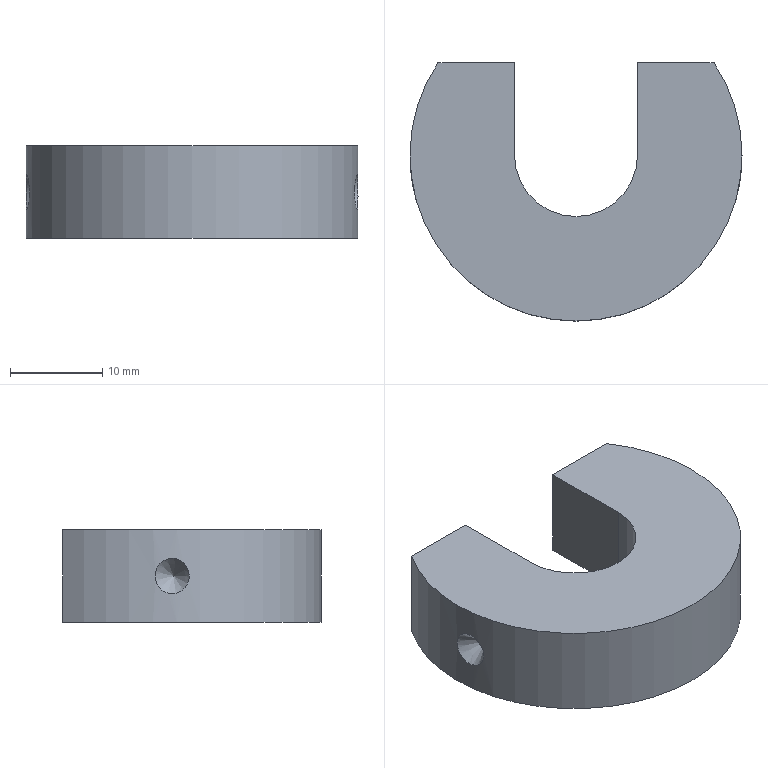Part | NX | features DATUM_CSYS 4, CONE 2, SKETCH 2, EXTRUDE 1, MIRROR_SET 1 | 1 solid | 10 faces | box 36.001 x 28 x 10 mm | volume 6442 mm3 | plane 6 | cylinder 2 | cone 2 | commonest cylinder face diameters 13.349 x1 36 x1
STEP:
#1=CARTESIAN_POINT('',(17.755,-2.958,3.471));
#2=VERTEX_POINT('',#1);
#3=CARTESIAN_POINT('',(17.578,-3.865,4.697));
#4=CARTESIAN_POINT('',(17.749,-3.086,3.311));
#5=CARTESIAN_POINT('',(17.958,-1.543,2.887));
#6=CARTESIAN_POINT('',(18.006,-0.1872,3.755));
#7=CARTESIAN_POINT('',(17.997,0.1688,5.305));
#8=CARTESIAN_POINT('',(18.004,-0.6057,6.698));
#9=CARTESIAN_POINT('',(17.894,-2.162,7.108));
#10=CARTESIAN_POINT('',(17.663,-3.5,6.241));
#11=CARTESIAN_POINT('',(17.578,-3.865,4.697));
#12=CARTESIAN_POINT('',(17.749,-3.086,3.311));
#13=CARTESIAN_POINT('',(17.958,-1.543,2.887));
#14=B_SPLINE_CURVE_WITH_KNOTS('',3,(#3,#4,#5,#6,#7,#8,#9,#10,#11,#12,#13),.UNSPECIFIED.,.T.,.F.,(1,1,1,1,1,1,1,1,1,1,1,1,1,1,1),(-0.00444,-0.00296,-0.00148,0.,0.00148,0.00296,0.00444,0.00592,0.0074,0.00888,0.01036,0.01184,0.01332,0.0148,0.01628),.UNSPECIFIED.);
#15=EDGE_CURVE('',#2,#2,#14,.T.);
#16=ORIENTED_EDGE('',*,*,#15,.F.);
#17=EDGE_LOOP('',(#16));
#18=FACE_BOUND('',#17,.T.);
#19=CARTESIAN_POINT('',(-17.755,-2.958,3.471));
#20=VERTEX_POINT('',#19);
#21=CARTESIAN_POINT('',(-17.958,-1.541,2.887));
#22=CARTESIAN_POINT('',(-17.748,-3.086,3.311));
#23=CARTESIAN_POINT('',(-17.578,-3.865,4.696));
#24=CARTESIAN_POINT('',(-17.663,-3.5,6.241));
#25=CARTESIAN_POINT('',(-17.893,-2.167,7.107));
#26=CARTESIAN_POINT('',(-18.004,-0.6063,6.7));
#27=CARTESIAN_POINT('',(-17.997,0.1689,5.305));
#28=CARTESIAN_POINT('',(-18.006,-0.1867,3.757));
#29=CARTESIAN_POINT('',(-17.958,-1.541,2.887));
#30=CARTESIAN_POINT('',(-17.748,-3.086,3.311));
#31=CARTESIAN_POINT('',(-17.578,-3.865,4.696));
#32=B_SPLINE_CURVE_WITH_KNOTS('',3,(#21,#22,#23,#24,#25,#26,#27,#28,#29,#30,#31),.UNSPECIFIED.,.T.,.F.,(1,1,1,1,1,1,1,1,1,1,1,1,1,1,1),(-0.004442,-0.002961,-0.001481,0.,0.001481,0.002961,0.004442,0.005922,0.007403,0.008884,0.01036,0.01184,0.01333,0.01481,0.01629),.UNSPECIFIED.);
#33=EDGE_CURVE('',#20,#20,#32,.T.);
#34=ORIENTED_EDGE('',*,*,#33,.F.);
#35=EDGE_LOOP('',(#34));
#36=FACE_BOUND('',#35,.T.);
#37=CARTESIAN_POINT('',(14.966,10.,0.));
#38=VERTEX_POINT('',#37);
#39=CARTESIAN_POINT('',(-14.966,10.,0.));
#40=VERTEX_POINT('',#39);
#41=CARTESIAN_POINT('',(0.,0.,0.));
#42=DIRECTION('',(0.,0.,-1.));
#43=DIRECTION('',(1.,0.,0.));
#44=AXIS2_PLACEMENT_3D('',#41,#42,#43);
#45=CIRCLE('',#44,18.);
#46=EDGE_CURVE('',#38,#40,#45,.T.);
#47=ORIENTED_EDGE('',*,*,#46,.F.);
#48=CARTESIAN_POINT('',(14.966,10.,10.));
#49=VERTEX_POINT('',#48);
#50=CARTESIAN_POINT('',(14.966,10.,10.));
#51=DIRECTION('',(0.,0.,-1.));
#52=VECTOR('',#51,1000.);
#53=LINE('',#50,#52);
#54=EDGE_CURVE('',#49,#38,#53,.T.);
#55=ORIENTED_EDGE('',*,*,#54,.F.);
#56=CARTESIAN_POINT('',(-14.966,10.,10.));
#57=VERTEX_POINT('',#56);
#58=CARTESIAN_POINT('',(0.,0.,10.));
#59=DIRECTION('',(0.,0.,-1.));
#60=DIRECTION('',(1.,0.,0.));
#61=AXIS2_PLACEMENT_3D('',#58,#59,#60);
#62=CIRCLE('',#61,18.);
#63=EDGE_CURVE('',#49,#57,#62,.T.);
#64=ORIENTED_EDGE('',*,*,#63,.T.);
#65=CARTESIAN_POINT('',(-14.966,10.,10.));
#66=DIRECTION('',(0.,0.,-1.));
#67=VECTOR('',#66,1000.);
#68=LINE('',#65,#67);
#69=EDGE_CURVE('',#57,#40,#68,.T.);
#70=ORIENTED_EDGE('',*,*,#69,.T.);
#71=EDGE_LOOP('',(#47,#55,#64,#70));
#72=FACE_BOUND('',#71,.T.);
#73=CARTESIAN_POINT('',(0.,0.,10.));
#74=DIRECTION('',(0.,0.,-1.));
#75=DIRECTION('',(-1.,0.,0.));
#76=AXIS2_PLACEMENT_3D('',#73,#74,#75);
#77=CYLINDRICAL_SURFACE('',#76,18.);
#78=ADVANCED_FACE('',(#18,#36,#72),#77,.T.);
#79=CARTESIAN_POINT('',(-6.675,10.,0.));
#80=VERTEX_POINT('',#79);
#81=CARTESIAN_POINT('',(-14.966,10.,0.));
#82=DIRECTION('',(1.,0.,0.));
#83=VECTOR('',#82,1000.);
#84=LINE('',#81,#83);
#85=EDGE_CURVE('',#40,#80,#84,.T.);
#86=ORIENTED_EDGE('',*,*,#85,.F.);
#87=ORIENTED_EDGE('',*,*,#69,.F.);
#88=CARTESIAN_POINT('',(-6.675,10.,10.));
#89=VERTEX_POINT('',#88);
#90=CARTESIAN_POINT('',(-14.966,10.,10.));
#91=DIRECTION('',(1.,0.,0.));
#92=VECTOR('',#91,1000.);
#93=LINE('',#90,#92);
#94=EDGE_CURVE('',#57,#89,#93,.T.);
#95=ORIENTED_EDGE('',*,*,#94,.T.);
#96=CARTESIAN_POINT('',(-6.675,10.,10.));
#97=DIRECTION('',(0.,0.,-1.));
#98=VECTOR('',#97,1000.);
#99=LINE('',#96,#98);
#100=EDGE_CURVE('',#89,#80,#99,.T.);
#101=ORIENTED_EDGE('',*,*,#100,.T.);
#102=EDGE_LOOP('',(#86,#87,#95,#101));
#103=FACE_BOUND('',#102,.T.);
#104=CARTESIAN_POINT('',(-14.966,10.,10.));
#105=DIRECTION('',(0.,1.,0.));
#106=DIRECTION('',(0.,0.,1.));
#107=AXIS2_PLACEMENT_3D('',#104,#105,#106);
#108=PLANE('',#107);
#109=ADVANCED_FACE('',(#103),#108,.T.);
#110=CARTESIAN_POINT('',(-6.675,0.,0.));
#111=VERTEX_POINT('',#110);
#112=CARTESIAN_POINT('',(-6.675,10.,0.));
#113=DIRECTION('',(0.,-1.,0.));
#114=VECTOR('',#113,1000.);
#115=LINE('',#112,#114);
#116=EDGE_CURVE('',#80,#111,#115,.T.);
#117=ORIENTED_EDGE('',*,*,#116,.F.);
#118=ORIENTED_EDGE('',*,*,#100,.F.);
#119=CARTESIAN_POINT('',(-6.675,0.,10.));
#120=VERTEX_POINT('',#119);
#121=CARTESIAN_POINT('',(-6.675,10.,10.));
#122=DIRECTION('',(0.,-1.,0.));
#123=VECTOR('',#122,1000.);
#124=LINE('',#121,#123);
#125=EDGE_CURVE('',#89,#120,#124,.T.);
#126=ORIENTED_EDGE('',*,*,#125,.T.);
#127=CARTESIAN_POINT('',(-6.675,0.,10.));
#128=DIRECTION('',(0.,0.,-1.));
#129=VECTOR('',#128,1000.);
#130=LINE('',#127,#129);
#131=EDGE_CURVE('',#120,#111,#130,.T.);
#132=ORIENTED_EDGE('',*,*,#131,.T.);
#133=EDGE_LOOP('',(#117,#118,#126,#132));
#134=FACE_BOUND('',#133,.T.);
#135=CARTESIAN_POINT('',(-6.675,10.,10.));
#136=DIRECTION('',(1.,0.,0.));
#137=DIRECTION('',(0.,1.,0.));
#138=AXIS2_PLACEMENT_3D('',#135,#136,#137);
#139=PLANE('',#138);
#140=ADVANCED_FACE('',(#134),#139,.T.);
#141=CARTESIAN_POINT('',(6.675,0.,0.));
#142=VERTEX_POINT('',#141);
#143=CARTESIAN_POINT('',(0.,0.,0.));
#144=DIRECTION('',(0.,0.,1.));
#145=DIRECTION('',(1.,0.,0.));
#146=AXIS2_PLACEMENT_3D('',#143,#144,#145);
#147=CIRCLE('',#146,6.675);
#148=EDGE_CURVE('',#111,#142,#147,.T.);
#149=ORIENTED_EDGE('',*,*,#148,.F.);
#150=ORIENTED_EDGE('',*,*,#131,.F.);
#151=CARTESIAN_POINT('',(6.675,0.,10.));
#152=VERTEX_POINT('',#151);
#153=CARTESIAN_POINT('',(0.,0.,10.));
#154=DIRECTION('',(0.,0.,1.));
#155=DIRECTION('',(1.,0.,0.));
#156=AXIS2_PLACEMENT_3D('',#153,#154,#155);
#157=CIRCLE('',#156,6.675);
#158=EDGE_CURVE('',#120,#152,#157,.T.);
#159=ORIENTED_EDGE('',*,*,#158,.T.);
#160=CARTESIAN_POINT('',(6.675,0.,10.));
#161=DIRECTION('',(0.,0.,-1.));
#162=VECTOR('',#161,1000.);
#163=LINE('',#160,#162);
#164=EDGE_CURVE('',#152,#142,#163,.T.);
#165=ORIENTED_EDGE('',*,*,#164,.T.);
#166=EDGE_LOOP('',(#149,#150,#159,#165));
#167=FACE_BOUND('',#166,.T.);
#168=CARTESIAN_POINT('',(0.,0.,10.));
#169=DIRECTION('',(0.,0.,-1.));
#170=DIRECTION('',(-1.,0.,0.));
#171=AXIS2_PLACEMENT_3D('',#168,#169,#170);
#172=CYLINDRICAL_SURFACE('',#171,6.675);
#173=ADVANCED_FACE('',(#167),#172,.F.);
#174=CARTESIAN_POINT('',(6.675,10.,0.));
#175=VERTEX_POINT('',#174);
#176=CARTESIAN_POINT('',(6.675,0.,0.));
#177=DIRECTION('',(0.,1.,0.));
#178=VECTOR('',#177,1000.);
#179=LINE('',#176,#178);
#180=EDGE_CURVE('',#142,#175,#179,.T.);
#181=ORIENTED_EDGE('',*,*,#180,.F.);
#182=ORIENTED_EDGE('',*,*,#164,.F.);
#183=CARTESIAN_POINT('',(6.675,10.,10.));
#184=VERTEX_POINT('',#183);
#185=CARTESIAN_POINT('',(6.675,0.,10.));
#186=DIRECTION('',(0.,1.,0.));
#187=VECTOR('',#186,1000.);
#188=LINE('',#185,#187);
#189=EDGE_CURVE('',#152,#184,#188,.T.);
#190=ORIENTED_EDGE('',*,*,#189,.T.);
#191=CARTESIAN_POINT('',(6.675,10.,10.));
#192=DIRECTION('',(0.,0.,-1.));
#193=VECTOR('',#192,1000.);
#194=LINE('',#191,#193);
#195=EDGE_CURVE('',#184,#175,#194,.T.);
#196=ORIENTED_EDGE('',*,*,#195,.T.);
#197=EDGE_LOOP('',(#181,#182,#190,#196));
#198=FACE_BOUND('',#197,.T.);
#199=CARTESIAN_POINT('',(6.675,0.,10.));
#200=DIRECTION('',(-1.,0.,0.));
#201=DIRECTION('',(0.,0.,1.));
#202=AXIS2_PLACEMENT_3D('',#199,#200,#201);
#203=PLANE('',#202);
#204=ADVANCED_FACE('',(#198),#203,.T.);
#205=CARTESIAN_POINT('',(6.675,10.,0.));
#206=DIRECTION('',(1.,0.,0.));
#207=VECTOR('',#206,1000.);
#208=LINE('',#205,#207);
#209=EDGE_CURVE('',#175,#38,#208,.T.);
#210=ORIENTED_EDGE('',*,*,#209,.F.);
#211=ORIENTED_EDGE('',*,*,#195,.F.);
#212=CARTESIAN_POINT('',(6.675,10.,10.));
#213=DIRECTION('',(1.,0.,0.));
#214=VECTOR('',#213,1000.);
#215=LINE('',#212,#214);
#216=EDGE_CURVE('',#184,#49,#215,.T.);
#217=ORIENTED_EDGE('',*,*,#216,.T.);
#218=ORIENTED_EDGE('',*,*,#54,.T.);
#219=EDGE_LOOP('',(#210,#211,#217,#218));
#220=FACE_BOUND('',#219,.T.);
#221=CARTESIAN_POINT('',(6.675,10.,10.));
#222=DIRECTION('',(0.,1.,0.));
#223=DIRECTION('',(0.,0.,1.));
#224=AXIS2_PLACEMENT_3D('',#221,#222,#223);
#225=PLANE('',#224);
#226=ADVANCED_FACE('',(#220),#225,.T.);
#227=ORIENTED_EDGE('',*,*,#63,.F.);
#228=ORIENTED_EDGE('',*,*,#216,.F.);
#229=ORIENTED_EDGE('',*,*,#189,.F.);
#230=ORIENTED_EDGE('',*,*,#158,.F.);
#231=ORIENTED_EDGE('',*,*,#125,.F.);
#232=ORIENTED_EDGE('',*,*,#94,.F.);
#233=EDGE_LOOP('',(#227,#228,#229,#230,#231,#232));
#234=FACE_BOUND('',#233,.T.);
#235=CARTESIAN_POINT('',(0.,0.,10.));
#236=DIRECTION('',(0.,0.,-1.));
#237=DIRECTION('',(-1.,0.,0.));
#238=AXIS2_PLACEMENT_3D('',#235,#236,#237);
#239=PLANE('',#238);
#240=ADVANCED_FACE('',(#234),#239,.F.);
#241=ORIENTED_EDGE('',*,*,#46,.T.);
#242=ORIENTED_EDGE('',*,*,#85,.T.);
#243=ORIENTED_EDGE('',*,*,#116,.T.);
#244=ORIENTED_EDGE('',*,*,#148,.T.);
#245=ORIENTED_EDGE('',*,*,#180,.T.);
#246=ORIENTED_EDGE('',*,*,#209,.T.);
#247=EDGE_LOOP('',(#241,#242,#243,#244,#245,#246));
#248=FACE_BOUND('',#247,.T.);
#249=CARTESIAN_POINT('',(0.,0.,0.));
#250=DIRECTION('',(0.,0.,-1.));
#251=DIRECTION('',(-1.,0.,0.));
#252=AXIS2_PLACEMENT_3D('',#249,#250,#251);
#253=PLANE('',#252);
#254=ADVANCED_FACE('',(#248),#253,.T.);
#255=ORIENTED_EDGE('',*,*,#33,.T.);
#256=EDGE_LOOP('',(#255));
#257=FACE_BOUND('',#256,.T.);
#258=CARTESIAN_POINT('',(-15.5,-2.,5.));
#259=VERTEX_POINT('',#258);
#260=VERTEX_LOOP('',#259);
#261=FACE_BOUND('',#260,.T.);
#262=CARTESIAN_POINT('',(-15.5,-2.,5.));
#263=DIRECTION('',(-1.,0.,0.));
#264=DIRECTION('',(0.,-1.,0.));
#265=AXIS2_PLACEMENT_3D('',#262,#263,#264);
#266=CONICAL_SURFACE('',#265,0.,0.6747);
#267=ADVANCED_FACE('',(#257,#261),#266,.F.);
#268=ORIENTED_EDGE('',*,*,#15,.T.);
#269=EDGE_LOOP('',(#268));
#270=FACE_BOUND('',#269,.T.);
#271=CARTESIAN_POINT('',(15.5,-2.,5.));
#272=VERTEX_POINT('',#271);
#273=VERTEX_LOOP('',#272);
#274=FACE_BOUND('',#273,.T.);
#275=CARTESIAN_POINT('',(15.5,-2.,5.));
#276=DIRECTION('',(1.,0.,0.));
#277=DIRECTION('',(0.,-1.,0.));
#278=AXIS2_PLACEMENT_3D('',#275,#276,#277);
#279=CONICAL_SURFACE('',#278,0.,0.6747);
#280=ADVANCED_FACE('',(#270,#274),#279,.F.);
#281=CLOSED_SHELL('',(#78,#109,#140,#173,#204,#226,#240,#254,#267,#280));
#282=MANIFOLD_SOLID_BREP('',#281);
#283=(LENGTH_UNIT()NAMED_UNIT(*)SI_UNIT(.MILLI.,.METRE.));
#284=UNCERTAINTY_MEASURE_WITH_UNIT(LENGTH_MEASURE(0.0508),#283,'','');
#285=(NAMED_UNIT(*)PLANE_ANGLE_UNIT()SI_UNIT($,.RADIAN.));
#286=(NAMED_UNIT(*)SI_UNIT($,.STERADIAN.)SOLID_ANGLE_UNIT());
#287=(GEOMETRIC_REPRESENTATION_CONTEXT(3)GLOBAL_UNCERTAINTY_ASSIGNED_CONTEXT((#284))GLOBAL_UNIT_ASSIGNED_CONTEXT((#283,#285,#286))REPRESENTATION_CONTEXT('',''));
#288=ADVANCED_BREP_SHAPE_REPRESENTATION('',(#282),#287);